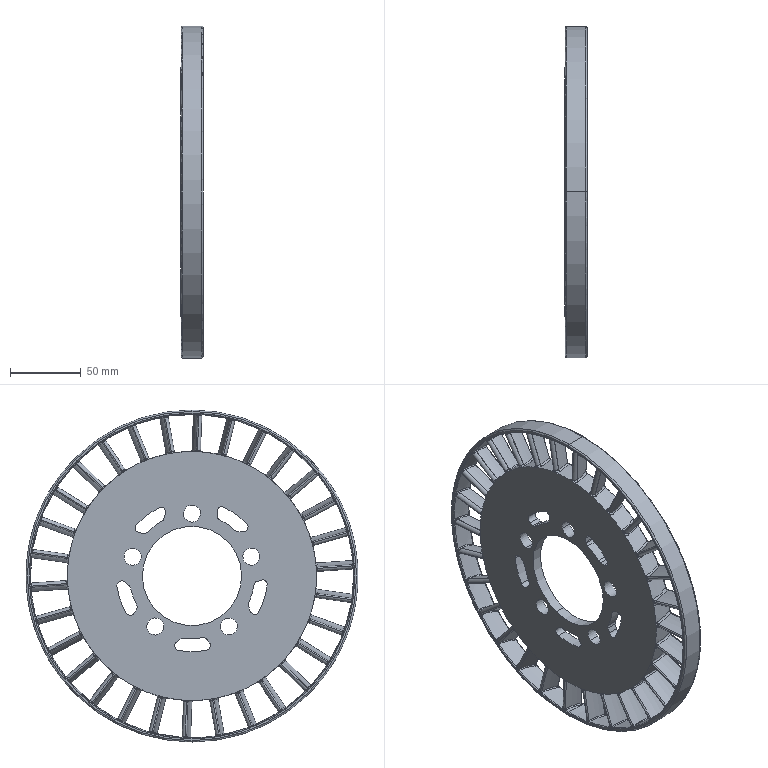Part | STEP file | Completa.sldasm-Part-19_Valor predeterminado | 1 solid | 949 faces | box 15.548 x 234.027 x 234.027 mm | volume 234749 mm3 | spline 540 | cylinder 321 | torus 73 | plane 15 | commonest cylinder face diameters 1.21 x60 4.84 x60 175.45 x31 228.027 x31 1.452 x30 64.773 x30